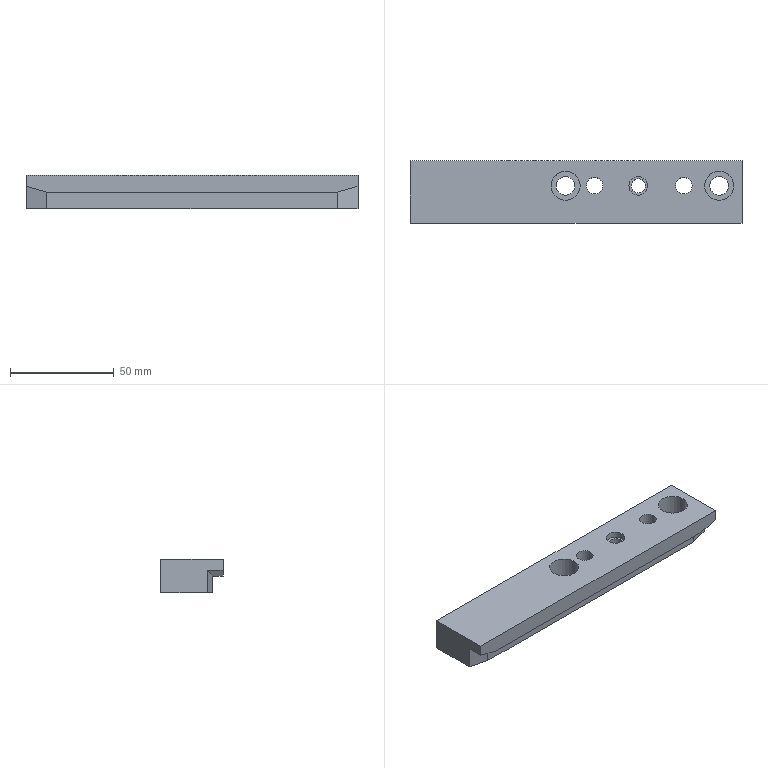Part | STEP file | lll_id4694_x_t | 1 solid | 23 faces | box 160 x 30 x 16 mm | volume 63890 mm3 | plane 15 | cylinder 8 | commonest cylinder face diameters 9 x3 8 x2 14 x2 6.8 x1
STEP:
#1=CARTESIAN_POINT('',(219.435,355.5,16.));
#2=VERTEX_POINT('',#1);
#3=CARTESIAN_POINT('',(212.435,355.5,16.));
#4=DIRECTION('',(0.,0.,-1.));
#5=DIRECTION('',(1.,0.,0.));
#6=AXIS2_PLACEMENT_3D('',#3,#4,#5);
#7=CIRCLE('',#6,7.);
#8=EDGE_CURVE('',#2,#2,#7,.T.);
#9=ORIENTED_EDGE('',*,*,#8,.T.);
#10=EDGE_LOOP('',(#9));
#11=FACE_BOUND('',#10,.T.);
#12=CARTESIAN_POINT('',(293.435,355.5,16.));
#13=VERTEX_POINT('',#12);
#14=CARTESIAN_POINT('',(286.435,355.5,16.));
#15=DIRECTION('',(0.,0.,1.));
#16=DIRECTION('',(1.,0.,0.));
#17=AXIS2_PLACEMENT_3D('',#14,#15,#16);
#18=CIRCLE('',#17,7.);
#19=EDGE_CURVE('',#13,#13,#18,.T.);
#20=ORIENTED_EDGE('',*,*,#19,.F.);
#21=EDGE_LOOP('',(#20));
#22=FACE_BOUND('',#21,.T.);
#23=CARTESIAN_POINT('',(230.435,355.5,16.));
#24=VERTEX_POINT('',#23);
#25=CARTESIAN_POINT('',(226.435,355.5,16.));
#26=DIRECTION('',(0.,0.,-1.));
#27=DIRECTION('',(1.,0.,0.));
#28=AXIS2_PLACEMENT_3D('',#25,#26,#27);
#29=CIRCLE('',#28,4.);
#30=EDGE_CURVE('',#24,#24,#29,.T.);
#31=ORIENTED_EDGE('',*,*,#30,.T.);
#32=EDGE_LOOP('',(#31));
#33=FACE_BOUND('',#32,.T.);
#34=CARTESIAN_POINT('',(273.435,355.5,16.));
#35=VERTEX_POINT('',#34);
#36=CARTESIAN_POINT('',(269.435,355.5,16.));
#37=DIRECTION('',(0.,0.,-1.));
#38=DIRECTION('',(1.,0.,0.));
#39=AXIS2_PLACEMENT_3D('',#36,#37,#38);
#40=CIRCLE('',#39,4.);
#41=EDGE_CURVE('',#35,#35,#40,.T.);
#42=ORIENTED_EDGE('',*,*,#41,.T.);
#43=EDGE_LOOP('',(#42));
#44=FACE_BOUND('',#43,.T.);
#45=CARTESIAN_POINT('',(297.435,367.5,16.));
#46=VERTEX_POINT('',#45);
#47=CARTESIAN_POINT('',(137.435,367.5,16.));
#48=VERTEX_POINT('',#47);
#49=CARTESIAN_POINT('',(297.435,367.5,16.));
#50=DIRECTION('',(-1.,0.,0.));
#51=VECTOR('',#50,1.);
#52=LINE('',#49,#51);
#53=EDGE_CURVE('',#46,#48,#52,.T.);
#54=ORIENTED_EDGE('',*,*,#53,.T.);
#55=CARTESIAN_POINT('',(137.435,337.5,16.));
#56=VERTEX_POINT('',#55);
#57=CARTESIAN_POINT('',(137.435,367.5,16.));
#58=DIRECTION('',(0.,-1.,0.));
#59=VECTOR('',#58,1.);
#60=LINE('',#57,#59);
#61=EDGE_CURVE('',#48,#56,#60,.T.);
#62=ORIENTED_EDGE('',*,*,#61,.T.);
#63=CARTESIAN_POINT('',(297.435,337.5,16.));
#64=VERTEX_POINT('',#63);
#65=CARTESIAN_POINT('',(217.435,337.5,16.));
#66=DIRECTION('',(1.,0.,0.));
#67=VECTOR('',#66,1.);
#68=LINE('',#65,#67);
#69=EDGE_CURVE('',#56,#64,#68,.T.);
#70=ORIENTED_EDGE('',*,*,#69,.T.);
#71=CARTESIAN_POINT('',(297.435,337.5,16.));
#72=DIRECTION('',(0.,1.,0.));
#73=VECTOR('',#72,1.);
#74=LINE('',#71,#73);
#75=EDGE_CURVE('',#64,#46,#74,.T.);
#76=ORIENTED_EDGE('',*,*,#75,.T.);
#77=EDGE_LOOP('',(#54,#62,#70,#76));
#78=FACE_BOUND('',#77,.T.);
#79=CARTESIAN_POINT('',(251.935,355.5,16.));
#80=VERTEX_POINT('',#79);
#81=CARTESIAN_POINT('',(247.435,355.5,16.));
#82=DIRECTION('',(0.,0.,1.));
#83=DIRECTION('',(1.,0.,0.));
#84=AXIS2_PLACEMENT_3D('',#81,#82,#83);
#85=CIRCLE('',#84,4.5);
#86=EDGE_CURVE('',#80,#80,#85,.T.);
#87=ORIENTED_EDGE('',*,*,#86,.F.);
#88=EDGE_LOOP('',(#87));
#89=FACE_BOUND('',#88,.T.);
#90=CARTESIAN_POINT('',(217.435,367.5,16.));
#91=DIRECTION('',(0.,0.,1.));
#92=DIRECTION('',(1.,0.,0.));
#93=AXIS2_PLACEMENT_3D('',#90,#91,#92);
#94=PLANE('',#93);
#95=ADVANCED_FACE('',(#11,#22,#33,#44,#78,#89),#94,.T.);
#96=CARTESIAN_POINT('',(216.935,355.5,0.));
#97=VERTEX_POINT('',#96);
#98=CARTESIAN_POINT('',(212.435,355.5,0.));
#99=DIRECTION('',(0.,0.,1.));
#100=DIRECTION('',(1.,0.,0.));
#101=AXIS2_PLACEMENT_3D('',#98,#99,#100);
#102=CIRCLE('',#101,4.5);
#103=EDGE_CURVE('',#97,#97,#102,.T.);
#104=ORIENTED_EDGE('',*,*,#103,.F.);
#105=EDGE_LOOP('',(#104));
#106=FACE_BOUND('',#105,.T.);
#107=CARTESIAN_POINT('',(216.935,355.5,6.));
#108=VERTEX_POINT('',#107);
#109=CARTESIAN_POINT('',(212.435,355.5,6.));
#110=DIRECTION('',(0.,0.,1.));
#111=DIRECTION('',(1.,0.,0.));
#112=AXIS2_PLACEMENT_3D('',#109,#110,#111);
#113=CIRCLE('',#112,4.5);
#114=EDGE_CURVE('',#108,#108,#113,.T.);
#115=ORIENTED_EDGE('',*,*,#114,.T.);
#116=EDGE_LOOP('',(#115));
#117=FACE_BOUND('',#116,.T.);
#118=CARTESIAN_POINT('',(212.435,355.5,47.));
#119=DIRECTION('',(0.,0.,-1.));
#120=DIRECTION('',(-1.,0.,0.));
#121=AXIS2_PLACEMENT_3D('',#118,#119,#120);
#122=CYLINDRICAL_SURFACE('',#121,4.5);
#123=ADVANCED_FACE('',(#106,#117),#122,.F.);
#124=CARTESIAN_POINT('',(230.435,355.5,0.));
#125=VERTEX_POINT('',#124);
#126=CARTESIAN_POINT('',(226.435,355.5,0.));
#127=DIRECTION('',(0.,0.,1.));
#128=DIRECTION('',(1.,0.,0.));
#129=AXIS2_PLACEMENT_3D('',#126,#127,#128);
#130=CIRCLE('',#129,4.);
#131=EDGE_CURVE('',#125,#125,#130,.T.);
#132=ORIENTED_EDGE('',*,*,#131,.T.);
#133=EDGE_LOOP('',(#132));
#134=FACE_BOUND('',#133,.T.);
#135=CARTESIAN_POINT('',(273.435,355.5,0.));
#136=VERTEX_POINT('',#135);
#137=CARTESIAN_POINT('',(269.435,355.5,0.));
#138=DIRECTION('',(0.,0.,1.));
#139=DIRECTION('',(1.,0.,0.));
#140=AXIS2_PLACEMENT_3D('',#137,#138,#139);
#141=CIRCLE('',#140,4.);
#142=EDGE_CURVE('',#136,#136,#141,.T.);
#143=ORIENTED_EDGE('',*,*,#142,.T.);
#144=EDGE_LOOP('',(#143));
#145=FACE_BOUND('',#144,.T.);
#146=CARTESIAN_POINT('',(137.435,345.18,0.));
#147=VERTEX_POINT('',#146);
#148=CARTESIAN_POINT('',(147.437,342.5,0.));
#149=VERTEX_POINT('',#148);
#150=CARTESIAN_POINT('',(137.435,345.18,0.));
#151=DIRECTION('',(0.9659,-0.2588,0.));
#152=VECTOR('',#151,1.);
#153=LINE('',#150,#152);
#154=EDGE_CURVE('',#147,#149,#153,.T.);
#155=ORIENTED_EDGE('',*,*,#154,.F.);
#156=CARTESIAN_POINT('',(137.435,367.5,0.));
#157=VERTEX_POINT('',#156);
#158=CARTESIAN_POINT('',(137.435,367.5,0.));
#159=DIRECTION('',(0.,-1.,0.));
#160=VECTOR('',#159,1.);
#161=LINE('',#158,#160);
#162=EDGE_CURVE('',#157,#147,#161,.T.);
#163=ORIENTED_EDGE('',*,*,#162,.F.);
#164=CARTESIAN_POINT('',(297.435,367.5,0.));
#165=VERTEX_POINT('',#164);
#166=CARTESIAN_POINT('',(297.435,367.5,0.));
#167=DIRECTION('',(-1.,0.,0.));
#168=VECTOR('',#167,1.);
#169=LINE('',#166,#168);
#170=EDGE_CURVE('',#165,#157,#169,.T.);
#171=ORIENTED_EDGE('',*,*,#170,.F.);
#172=CARTESIAN_POINT('',(297.435,345.179,0.));
#173=VERTEX_POINT('',#172);
#174=CARTESIAN_POINT('',(297.435,337.5,0.));
#175=DIRECTION('',(0.,1.,0.));
#176=VECTOR('',#175,1.);
#177=LINE('',#174,#176);
#178=EDGE_CURVE('',#173,#165,#177,.T.);
#179=ORIENTED_EDGE('',*,*,#178,.F.);
#180=CARTESIAN_POINT('',(287.436,342.5,0.));
#181=VERTEX_POINT('',#180);
#182=CARTESIAN_POINT('',(287.436,342.5,0.));
#183=DIRECTION('',(0.9659,0.2588,0.));
#184=VECTOR('',#183,1.);
#185=LINE('',#182,#184);
#186=EDGE_CURVE('',#181,#173,#185,.T.);
#187=ORIENTED_EDGE('',*,*,#186,.F.);
#188=CARTESIAN_POINT('',(227.437,342.5,0.));
#189=DIRECTION('',(1.,0.,0.));
#190=VECTOR('',#189,1.);
#191=LINE('',#188,#190);
#192=EDGE_CURVE('',#149,#181,#191,.T.);
#193=ORIENTED_EDGE('',*,*,#192,.F.);
#194=EDGE_LOOP('',(#155,#163,#171,#179,#187,#193));
#195=FACE_BOUND('',#194,.T.);
#196=CARTESIAN_POINT('',(290.935,355.5,0.));
#197=VERTEX_POINT('',#196);
#198=CARTESIAN_POINT('',(286.435,355.5,0.));
#199=DIRECTION('',(0.,0.,1.));
#200=DIRECTION('',(1.,0.,0.));
#201=AXIS2_PLACEMENT_3D('',#198,#199,#200);
#202=CIRCLE('',#201,4.5);
#203=EDGE_CURVE('',#197,#197,#202,.T.);
#204=ORIENTED_EDGE('',*,*,#203,.T.);
#205=EDGE_LOOP('',(#204));
#206=FACE_BOUND('',#205,.T.);
#207=CARTESIAN_POINT('',(250.835,355.5,0.));
#208=VERTEX_POINT('',#207);
#209=CARTESIAN_POINT('',(247.435,355.5,0.));
#210=DIRECTION('',(0.,0.,1.));
#211=DIRECTION('',(1.,0.,0.));
#212=AXIS2_PLACEMENT_3D('',#209,#210,#211);
#213=CIRCLE('',#212,3.4);
#214=EDGE_CURVE('',#208,#208,#213,.T.);
#215=ORIENTED_EDGE('',*,*,#214,.T.);
#216=EDGE_LOOP('',(#215));
#217=FACE_BOUND('',#216,.T.);
#218=ORIENTED_EDGE('',*,*,#103,.T.);
#219=EDGE_LOOP('',(#218));
#220=FACE_BOUND('',#219,.T.);
#221=CARTESIAN_POINT('',(217.435,367.5,0.));
#222=DIRECTION('',(0.,0.,1.));
#223=DIRECTION('',(1.,0.,0.));
#224=AXIS2_PLACEMENT_3D('',#221,#222,#223);
#225=PLANE('',#224);
#226=ADVANCED_FACE('',(#134,#145,#195,#206,#217,#220),#225,.F.);
#227=ORIENTED_EDGE('',*,*,#170,.T.);
#228=CARTESIAN_POINT('',(137.435,367.5,16.));
#229=DIRECTION('',(0.,0.,-1.));
#230=VECTOR('',#229,1.);
#231=LINE('',#228,#230);
#232=EDGE_CURVE('',#48,#157,#231,.T.);
#233=ORIENTED_EDGE('',*,*,#232,.F.);
#234=ORIENTED_EDGE('',*,*,#53,.F.);
#235=CARTESIAN_POINT('',(297.435,367.5,16.));
#236=DIRECTION('',(0.,0.,-1.));
#237=VECTOR('',#236,1.);
#238=LINE('',#235,#237);
#239=EDGE_CURVE('',#46,#165,#238,.T.);
#240=ORIENTED_EDGE('',*,*,#239,.T.);
#241=EDGE_LOOP('',(#227,#233,#234,#240));
#242=FACE_OUTER_BOUND('',#241,.T.);
#243=CARTESIAN_POINT('',(297.435,367.5,16.));
#244=DIRECTION('',(0.,-1.,0.));
#245=DIRECTION('',(0.,0.,-1.));
#246=AXIS2_PLACEMENT_3D('',#243,#244,#245);
#247=PLANE('',#246);
#248=ADVANCED_FACE('',(#242),#247,.F.);
#249=CARTESIAN_POINT('',(137.435,345.18,10.679));
#250=VERTEX_POINT('',#249);
#251=CARTESIAN_POINT('',(137.435,345.18,8.));
#252=DIRECTION('',(0.,0.,-1.));
#253=VECTOR('',#252,1.);
#254=LINE('',#251,#253);
#255=EDGE_CURVE('',#250,#147,#254,.T.);
#256=ORIENTED_EDGE('',*,*,#255,.F.);
#257=CARTESIAN_POINT('',(137.435,337.5,10.679));
#258=VERTEX_POINT('',#257);
#259=CARTESIAN_POINT('',(137.435,367.5,10.679));
#260=DIRECTION('',(0.,-1.,0.));
#261=VECTOR('',#260,1.);
#262=LINE('',#259,#261);
#263=EDGE_CURVE('',#250,#258,#262,.T.);
#264=ORIENTED_EDGE('',*,*,#263,.T.);
#265=CARTESIAN_POINT('',(137.435,337.5,16.));
#266=DIRECTION('',(0.,0.,-1.));
#267=VECTOR('',#266,1.);
#268=LINE('',#265,#267);
#269=EDGE_CURVE('',#56,#258,#268,.T.);
#270=ORIENTED_EDGE('',*,*,#269,.F.);
#271=ORIENTED_EDGE('',*,*,#61,.F.);
#272=ORIENTED_EDGE('',*,*,#232,.T.);
#273=ORIENTED_EDGE('',*,*,#162,.T.);
#274=EDGE_LOOP('',(#256,#264,#270,#271,#272,#273));
#275=FACE_OUTER_BOUND('',#274,.T.);
#276=CARTESIAN_POINT('',(137.435,367.5,16.));
#277=DIRECTION('',(1.,0.,0.));
#278=DIRECTION('',(0.,0.,-1.));
#279=AXIS2_PLACEMENT_3D('',#276,#277,#278);
#280=PLANE('',#279);
#281=ADVANCED_FACE('',(#275),#280,.F.);
#282=ORIENTED_EDGE('',*,*,#269,.T.);
#283=CARTESIAN_POINT('',(147.435,337.5,8.));
#284=VERTEX_POINT('',#283);
#285=CARTESIAN_POINT('',(137.435,337.5,10.679));
#286=DIRECTION('',(0.9659,0.,-0.2588));
#287=VECTOR('',#286,1.);
#288=LINE('',#285,#287);
#289=EDGE_CURVE('',#258,#284,#288,.T.);
#290=ORIENTED_EDGE('',*,*,#289,.T.);
#291=CARTESIAN_POINT('',(287.435,337.5,8.));
#292=VERTEX_POINT('',#291);
#293=CARTESIAN_POINT('',(217.435,337.5,8.));
#294=DIRECTION('',(1.,0.,0.));
#295=VECTOR('',#294,1.);
#296=LINE('',#293,#295);
#297=EDGE_CURVE('',#284,#292,#296,.T.);
#298=ORIENTED_EDGE('',*,*,#297,.T.);
#299=CARTESIAN_POINT('',(297.435,337.5,10.679));
#300=VERTEX_POINT('',#299);
#301=CARTESIAN_POINT('',(297.435,337.5,10.679));
#302=DIRECTION('',(0.9659,0.,0.2588));
#303=VECTOR('',#302,1.);
#304=LINE('',#301,#303);
#305=EDGE_CURVE('',#292,#300,#304,.T.);
#306=ORIENTED_EDGE('',*,*,#305,.T.);
#307=CARTESIAN_POINT('',(297.435,337.5,16.));
#308=DIRECTION('',(0.,0.,-1.));
#309=VECTOR('',#308,1.);
#310=LINE('',#307,#309);
#311=EDGE_CURVE('',#64,#300,#310,.T.);
#312=ORIENTED_EDGE('',*,*,#311,.F.);
#313=ORIENTED_EDGE('',*,*,#69,.F.);
#314=EDGE_LOOP('',(#282,#290,#298,#306,#312,#313));
#315=FACE_OUTER_BOUND('',#314,.T.);
#316=CARTESIAN_POINT('',(217.435,337.5,16.));
#317=DIRECTION('',(0.,1.,0.));
#318=DIRECTION('',(0.,0.,1.));
#319=AXIS2_PLACEMENT_3D('',#316,#317,#318);
#320=PLANE('',#319);
#321=ADVANCED_FACE('',(#315),#320,.F.);
#322=ORIENTED_EDGE('',*,*,#311,.T.);
#323=CARTESIAN_POINT('',(297.435,345.179,10.679));
#324=VERTEX_POINT('',#323);
#325=CARTESIAN_POINT('',(297.435,337.5,10.679));
#326=DIRECTION('',(0.,1.,0.));
#327=VECTOR('',#326,1.);
#328=LINE('',#325,#327);
#329=EDGE_CURVE('',#300,#324,#328,.T.);
#330=ORIENTED_EDGE('',*,*,#329,.T.);
#331=CARTESIAN_POINT('',(297.435,345.179,8.));
#332=DIRECTION('',(0.,0.,-1.));
#333=VECTOR('',#332,1.);
#334=LINE('',#331,#333);
#335=EDGE_CURVE('',#324,#173,#334,.T.);
#336=ORIENTED_EDGE('',*,*,#335,.T.);
#337=ORIENTED_EDGE('',*,*,#178,.T.);
#338=ORIENTED_EDGE('',*,*,#239,.F.);
#339=ORIENTED_EDGE('',*,*,#75,.F.);
#340=EDGE_LOOP('',(#322,#330,#336,#337,#338,#339));
#341=FACE_OUTER_BOUND('',#340,.T.);
#342=CARTESIAN_POINT('',(297.435,337.5,16.));
#343=DIRECTION('',(-1.,0.,0.));
#344=DIRECTION('',(0.,0.,1.));
#345=AXIS2_PLACEMENT_3D('',#342,#343,#344);
#346=PLANE('',#345);
#347=ADVANCED_FACE('',(#341),#346,.F.);
#348=ORIENTED_EDGE('',*,*,#297,.F.);
#349=CARTESIAN_POINT('',(147.435,342.501,8.));
#350=VERTEX_POINT('',#349);
#351=CARTESIAN_POINT('',(147.435,324.702,8.));
#352=DIRECTION('',(0.,1.,0.));
#353=VECTOR('',#352,1.);
#354=LINE('',#351,#353);
#355=EDGE_CURVE('',#284,#350,#354,.T.);
#356=ORIENTED_EDGE('',*,*,#355,.T.);
#357=CARTESIAN_POINT('',(147.437,342.5,8.));
#358=VERTEX_POINT('',#357);
#359=CARTESIAN_POINT('',(137.435,345.18,8.));
#360=DIRECTION('',(-0.9659,0.2588,0.));
#361=VECTOR('',#360,1.);
#362=LINE('',#359,#361);
#363=EDGE_CURVE('',#358,#350,#362,.T.);
#364=ORIENTED_EDGE('',*,*,#363,.F.);
#365=CARTESIAN_POINT('',(287.435,342.5,8.));
#366=VERTEX_POINT('',#365);
#367=CARTESIAN_POINT('',(227.437,342.5,8.));
#368=DIRECTION('',(-1.,0.,0.));
#369=VECTOR('',#368,1.);
#370=LINE('',#367,#369);
#371=EDGE_CURVE('',#366,#358,#370,.T.);
#372=ORIENTED_EDGE('',*,*,#371,.F.);
#373=CARTESIAN_POINT('',(287.435,324.702,8.));
#374=DIRECTION('',(0.,-1.,0.));
#375=VECTOR('',#374,1.);
#376=LINE('',#373,#375);
#377=EDGE_CURVE('',#366,#292,#376,.T.);
#378=ORIENTED_EDGE('',*,*,#377,.T.);
#379=EDGE_LOOP('',(#348,#356,#364,#372,#378));
#380=FACE_OUTER_BOUND('',#379,.T.);
#381=CARTESIAN_POINT('',(322.025,324.702,8.));
#382=DIRECTION('',(0.,0.,1.));
#383=DIRECTION('',(1.,0.,0.));
#384=AXIS2_PLACEMENT_3D('',#381,#382,#383);
#385=PLANE('',#384);
#386=ADVANCED_FACE('',(#380),#385,.F.);
#387=ORIENTED_EDGE('',*,*,#154,.T.);
#388=CARTESIAN_POINT('',(147.437,342.5,8.));
#389=DIRECTION('',(0.,0.,1.));
#390=VECTOR('',#389,1.);
#391=LINE('',#388,#390);
#392=EDGE_CURVE('',#149,#358,#391,.T.);
#393=ORIENTED_EDGE('',*,*,#392,.T.);
#394=ORIENTED_EDGE('',*,*,#363,.T.);
#395=CARTESIAN_POINT('',(138.063,345.012,10.511));
#396=DIRECTION('',(-0.9351,0.2506,0.2506));
#397=VECTOR('',#396,1.);
#398=LINE('',#395,#397);
#399=EDGE_CURVE('',#350,#250,#398,.T.);
#400=ORIENTED_EDGE('',*,*,#399,.T.);
#401=ORIENTED_EDGE('',*,*,#255,.T.);
#402=EDGE_LOOP('',(#387,#393,#394,#400,#401));
#403=FACE_OUTER_BOUND('',#402,.T.);
#404=CARTESIAN_POINT('',(137.435,345.18,8.));
#405=DIRECTION('',(0.2588,0.9659,0.));
#406=DIRECTION('',(-0.9659,0.2588,0.));
#407=AXIS2_PLACEMENT_3D('',#404,#405,#406);
#408=PLANE('',#407);
#409=ADVANCED_FACE('',(#403),#408,.F.);
#410=ORIENTED_EDGE('',*,*,#192,.T.);
#411=CARTESIAN_POINT('',(287.436,342.5,8.));
#412=VERTEX_POINT('',#411);
#413=CARTESIAN_POINT('',(287.436,342.5,8.));
#414=DIRECTION('',(0.,0.,1.));
#415=VECTOR('',#414,1.);
#416=LINE('',#413,#415);
#417=EDGE_CURVE('',#181,#412,#416,.T.);
#418=ORIENTED_EDGE('',*,*,#417,.T.);
#419=CARTESIAN_POINT('',(231.456,342.5,-7.));
#420=DIRECTION('',(-0.9659,0.,-0.2588));
#421=VECTOR('',#420,1.);
#422=LINE('',#419,#421);
#423=EDGE_CURVE('',#412,#366,#422,.T.);
#424=ORIENTED_EDGE('',*,*,#423,.T.);
#425=ORIENTED_EDGE('',*,*,#371,.T.);
#426=ORIENTED_EDGE('',*,*,#392,.F.);
#427=EDGE_LOOP('',(#410,#418,#424,#425,#426));
#428=FACE_OUTER_BOUND('',#427,.T.);
#429=CARTESIAN_POINT('',(227.437,342.5,8.));
#430=DIRECTION('',(0.,1.,0.));
#431=DIRECTION('',(0.,0.,1.));
#432=AXIS2_PLACEMENT_3D('',#429,#430,#431);
#433=PLANE('',#432);
#434=ADVANCED_FACE('',(#428),#433,.F.);
#435=ORIENTED_EDGE('',*,*,#186,.T.);
#436=ORIENTED_EDGE('',*,*,#335,.F.);
#437=CARTESIAN_POINT('',(287.436,342.5,8.));
#438=DIRECTION('',(-0.9351,-0.2506,-0.2506));
#439=VECTOR('',#438,1.);
#440=LINE('',#437,#439);
#441=EDGE_CURVE('',#324,#412,#440,.T.);
#442=ORIENTED_EDGE('',*,*,#441,.T.);
#443=ORIENTED_EDGE('',*,*,#417,.F.);
#444=EDGE_LOOP('',(#435,#436,#442,#443));
#445=FACE_OUTER_BOUND('',#444,.T.);
#446=CARTESIAN_POINT('',(287.436,342.5,8.));
#447=DIRECTION('',(-0.2588,0.9659,0.));
#448=DIRECTION('',(-0.9659,-0.2588,0.));
#449=AXIS2_PLACEMENT_3D('',#446,#447,#448);
#450=PLANE('',#449);
#451=ADVANCED_FACE('',(#445),#450,.F.);
#452=CARTESIAN_POINT('',(281.935,355.5,6.));
#453=VERTEX_POINT('',#452);
#454=CARTESIAN_POINT('',(286.435,355.5,6.));
#455=DIRECTION('',(0.,0.,-1.));
#456=DIRECTION('',(-1.,0.,0.));
#457=AXIS2_PLACEMENT_3D('',#454,#455,#456);
#458=CIRCLE('',#457,4.5);
#459=EDGE_CURVE('',#453,#453,#458,.T.);
#460=ORIENTED_EDGE('',*,*,#459,.F.);
#461=EDGE_LOOP('',(#460));
#462=FACE_BOUND('',#461,.T.);
#463=ORIENTED_EDGE('',*,*,#203,.F.);
#464=EDGE_LOOP('',(#463));
#465=FACE_BOUND('',#464,.T.);
#466=CARTESIAN_POINT('',(286.435,355.5,47.));
#467=DIRECTION('',(0.,0.,-1.));
#468=DIRECTION('',(-1.,0.,0.));
#469=AXIS2_PLACEMENT_3D('',#466,#467,#468);
#470=CYLINDRICAL_SURFACE('',#469,4.5);
#471=ADVANCED_FACE('',(#462,#465),#470,.F.);
#472=ORIENTED_EDGE('',*,*,#41,.F.);
#473=EDGE_LOOP('',(#472));
#474=FACE_BOUND('',#473,.T.);
#475=ORIENTED_EDGE('',*,*,#142,.F.);
#476=EDGE_LOOP('',(#475));
#477=FACE_BOUND('',#476,.T.);
#478=CARTESIAN_POINT('',(269.435,355.5,47.));
#479=DIRECTION('',(0.,0.,-1.));
#480=DIRECTION('',(-1.,0.,0.));
#481=AXIS2_PLACEMENT_3D('',#478,#479,#480);
#482=CYLINDRICAL_SURFACE('',#481,4.);
#483=ADVANCED_FACE('',(#474,#477),#482,.F.);
#484=CARTESIAN_POINT('',(244.035,355.5,13.));
#485=VERTEX_POINT('',#484);
#486=CARTESIAN_POINT('',(247.435,355.5,13.));
#487=DIRECTION('',(0.,0.,-1.));
#488=DIRECTION('',(-1.,0.,0.));
#489=AXIS2_PLACEMENT_3D('',#486,#487,#488);
#490=CIRCLE('',#489,3.4);
#491=EDGE_CURVE('',#485,#485,#490,.T.);
#492=ORIENTED_EDGE('',*,*,#491,.F.);
#493=EDGE_LOOP('',(#492));
#494=FACE_BOUND('',#493,.T.);
#495=ORIENTED_EDGE('',*,*,#214,.F.);
#496=EDGE_LOOP('',(#495));
#497=FACE_BOUND('',#496,.T.);
#498=CARTESIAN_POINT('',(247.435,355.5,47.));
#499=DIRECTION('',(0.,0.,-1.));
#500=DIRECTION('',(-1.,0.,0.));
#501=AXIS2_PLACEMENT_3D('',#498,#499,#500);
#502=CYLINDRICAL_SURFACE('',#501,3.4);
#503=ADVANCED_FACE('',(#494,#497),#502,.F.);
#504=ORIENTED_EDGE('',*,*,#30,.F.);
#505=EDGE_LOOP('',(#504));
#506=FACE_BOUND('',#505,.T.);
#507=ORIENTED_EDGE('',*,*,#131,.F.);
#508=EDGE_LOOP('',(#507));
#509=FACE_BOUND('',#508,.T.);
#510=CARTESIAN_POINT('',(226.435,355.5,47.));
#511=DIRECTION('',(0.,0.,-1.));
#512=DIRECTION('',(-1.,0.,0.));
#513=AXIS2_PLACEMENT_3D('',#510,#511,#512);
#514=CYLINDRICAL_SURFACE('',#513,4.);
#515=ADVANCED_FACE('',(#506,#509),#514,.F.);
#516=ORIENTED_EDGE('',*,*,#19,.T.);
#517=EDGE_LOOP('',(#516));
#518=FACE_BOUND('',#517,.T.);
#519=CARTESIAN_POINT('',(293.435,355.5,6.));
#520=VERTEX_POINT('',#519);
#521=CARTESIAN_POINT('',(286.435,355.5,6.));
#522=DIRECTION('',(0.,0.,1.));
#523=DIRECTION('',(1.,0.,0.));
#524=AXIS2_PLACEMENT_3D('',#521,#522,#523);
#525=CIRCLE('',#524,7.);
#526=EDGE_CURVE('',#520,#520,#525,.T.);
#527=ORIENTED_EDGE('',*,*,#526,.F.);
#528=EDGE_LOOP('',(#527));
#529=FACE_BOUND('',#528,.T.);
#530=CARTESIAN_POINT('',(286.435,355.5,47.));
#531=DIRECTION('',(0.,0.,-1.));
#532=DIRECTION('',(-1.,0.,0.));
#533=AXIS2_PLACEMENT_3D('',#530,#531,#532);
#534=CYLINDRICAL_SURFACE('',#533,7.);
#535=ADVANCED_FACE('',(#518,#529),#534,.F.);
#536=ORIENTED_EDGE('',*,*,#459,.T.);
#537=EDGE_LOOP('',(#536));
#538=FACE_BOUND('',#537,.T.);
#539=ORIENTED_EDGE('',*,*,#526,.T.);
#540=EDGE_LOOP('',(#539));
#541=FACE_BOUND('',#540,.T.);
#542=CARTESIAN_POINT('',(286.435,355.5,6.));
#543=DIRECTION('',(0.,0.,-1.));
#544=DIRECTION('',(-1.,0.,0.));
#545=AXIS2_PLACEMENT_3D('',#542,#543,#544);
#546=PLANE('',#545);
#547=ADVANCED_FACE('',(#538,#541),#546,.F.);
#548=ORIENTED_EDGE('',*,*,#8,.F.);
#549=EDGE_LOOP('',(#548));
#550=FACE_BOUND('',#549,.T.);
#551=CARTESIAN_POINT('',(219.435,355.5,6.));
#552=VERTEX_POINT('',#551);
#553=CARTESIAN_POINT('',(212.435,355.5,6.));
#554=DIRECTION('',(0.,0.,-1.));
#555=DIRECTION('',(1.,0.,0.));
#556=AXIS2_PLACEMENT_3D('',#553,#554,#555);
#557=CIRCLE('',#556,7.);
#558=EDGE_CURVE('',#552,#552,#557,.T.);
#559=ORIENTED_EDGE('',*,*,#558,.T.);
#560=EDGE_LOOP('',(#559));
#561=FACE_BOUND('',#560,.T.);
#562=CARTESIAN_POINT('',(212.435,355.5,47.));
#563=DIRECTION('',(0.,0.,-1.));
#564=DIRECTION('',(-1.,0.,0.));
#565=AXIS2_PLACEMENT_3D('',#562,#563,#564);
#566=CYLINDRICAL_SURFACE('',#565,7.);
#567=ADVANCED_FACE('',(#550,#561),#566,.F.);
#568=ORIENTED_EDGE('',*,*,#114,.F.);
#569=EDGE_LOOP('',(#568));
#570=FACE_BOUND('',#569,.T.);
#571=ORIENTED_EDGE('',*,*,#558,.F.);
#572=EDGE_LOOP('',(#571));
#573=FACE_BOUND('',#572,.T.);
#574=CARTESIAN_POINT('',(212.435,355.5,6.));
#575=DIRECTION('',(0.,0.,1.));
#576=DIRECTION('',(1.,0.,0.));
#577=AXIS2_PLACEMENT_3D('',#574,#575,#576);
#578=PLANE('',#577);
#579=ADVANCED_FACE('',(#570,#573),#578,.T.);
#580=ORIENTED_EDGE('',*,*,#86,.T.);
#581=EDGE_LOOP('',(#580));
#582=FACE_BOUND('',#581,.T.);
#583=CARTESIAN_POINT('',(251.935,355.5,13.));
#584=VERTEX_POINT('',#583);
#585=CARTESIAN_POINT('',(247.435,355.5,13.));
#586=DIRECTION('',(0.,0.,1.));
#587=DIRECTION('',(1.,0.,0.));
#588=AXIS2_PLACEMENT_3D('',#585,#586,#587);
#589=CIRCLE('',#588,4.5);
#590=EDGE_CURVE('',#584,#584,#589,.T.);
#591=ORIENTED_EDGE('',*,*,#590,.F.);
#592=EDGE_LOOP('',(#591));
#593=FACE_BOUND('',#592,.T.);
#594=CARTESIAN_POINT('',(247.435,355.5,47.));
#595=DIRECTION('',(0.,0.,-1.));
#596=DIRECTION('',(-1.,0.,0.));
#597=AXIS2_PLACEMENT_3D('',#594,#595,#596);
#598=CYLINDRICAL_SURFACE('',#597,4.5);
#599=ADVANCED_FACE('',(#582,#593),#598,.F.);
#600=ORIENTED_EDGE('',*,*,#491,.T.);
#601=EDGE_LOOP('',(#600));
#602=FACE_BOUND('',#601,.T.);
#603=ORIENTED_EDGE('',*,*,#590,.T.);
#604=EDGE_LOOP('',(#603));
#605=FACE_BOUND('',#604,.T.);
#606=CARTESIAN_POINT('',(247.435,355.5,13.));
#607=DIRECTION('',(0.,0.,-1.));
#608=DIRECTION('',(-1.,0.,0.));
#609=AXIS2_PLACEMENT_3D('',#606,#607,#608);
#610=PLANE('',#609);
#611=ADVANCED_FACE('',(#602,#605),#610,.F.);
#612=ORIENTED_EDGE('',*,*,#399,.F.);
#613=ORIENTED_EDGE('',*,*,#355,.F.);
#614=ORIENTED_EDGE('',*,*,#289,.F.);
#615=ORIENTED_EDGE('',*,*,#263,.F.);
#616=EDGE_LOOP('',(#612,#613,#614,#615));
#617=FACE_OUTER_BOUND('',#616,.T.);
#618=CARTESIAN_POINT('',(137.435,367.5,10.679));
#619=DIRECTION('',(0.2588,0.,0.9659));
#620=DIRECTION('',(0.9659,0.,-0.2588));
#621=AXIS2_PLACEMENT_3D('',#618,#619,#620);
#622=PLANE('',#621);
#623=ADVANCED_FACE('',(#617),#622,.F.);
#624=ORIENTED_EDGE('',*,*,#305,.F.);
#625=ORIENTED_EDGE('',*,*,#377,.F.);
#626=ORIENTED_EDGE('',*,*,#423,.F.);
#627=ORIENTED_EDGE('',*,*,#441,.F.);
#628=ORIENTED_EDGE('',*,*,#329,.F.);
#629=EDGE_LOOP('',(#624,#625,#626,#627,#628));
#630=FACE_OUTER_BOUND('',#629,.T.);
#631=CARTESIAN_POINT('',(297.435,337.5,10.679));
#632=DIRECTION('',(-0.2588,0.,0.9659));
#633=DIRECTION('',(0.9659,0.,0.2588));
#634=AXIS2_PLACEMENT_3D('',#631,#632,#633);
#635=PLANE('',#634);
#636=ADVANCED_FACE('',(#630),#635,.F.);
#637=CLOSED_SHELL('',(#95,#123,#226,#248,#281,#321,#347,#386,#409,#434,#451,#471,#483,#503,#515,#535,#547,#567,#579,#599,#611,#623,#636));
#638=MANIFOLD_SOLID_BREP('',#637);
#639=(LENGTH_UNIT()NAMED_UNIT(*)SI_UNIT(.MILLI.,.METRE.));
#640=UNCERTAINTY_MEASURE_WITH_UNIT(LENGTH_MEASURE(0.00002),#639,'','');
#641=(NAMED_UNIT(*)PLANE_ANGLE_UNIT()SI_UNIT($,.RADIAN.));
#642=PLANE_ANGLE_MEASURE_WITH_UNIT(PLANE_ANGLE_MEASURE(0.01745),#641);
#643=DIMENSIONAL_EXPONENTS(0.,0.,0.,0.,0.,0.,0.);
#644=(CONVERSION_BASED_UNIT('DEGREE',#642)NAMED_UNIT(#643)PLANE_ANGLE_UNIT());
#645=(NAMED_UNIT(*)SI_UNIT($,.STERADIAN.)SOLID_ANGLE_UNIT());
#646=(GEOMETRIC_REPRESENTATION_CONTEXT(3)GLOBAL_UNCERTAINTY_ASSIGNED_CONTEXT((#640))GLOBAL_UNIT_ASSIGNED_CONTEXT((#639,#644,#645))REPRESENTATION_CONTEXT('',''));
#647=ADVANCED_BREP_SHAPE_REPRESENTATION('',(#638),#646);